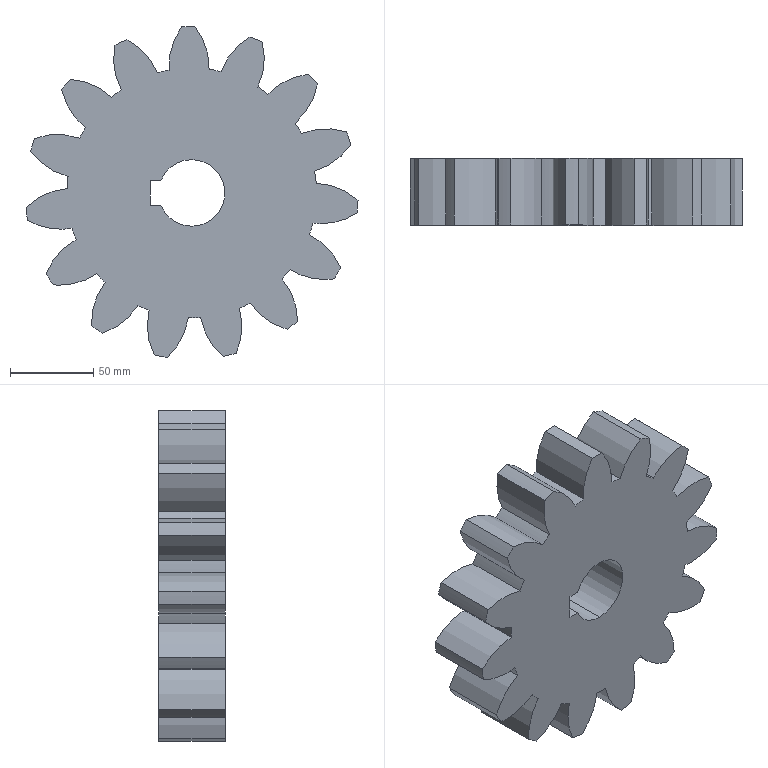Part | SolidWorks | features Extrusion 1 | 1 solid | 73 faces | box 199.536 x 40 x 198.904 mm | volume 944330 mm3 | cylinder 68 | plane 5 | commonest cylinder face diameters 80 x34 150 x16 200 x15 40 x3